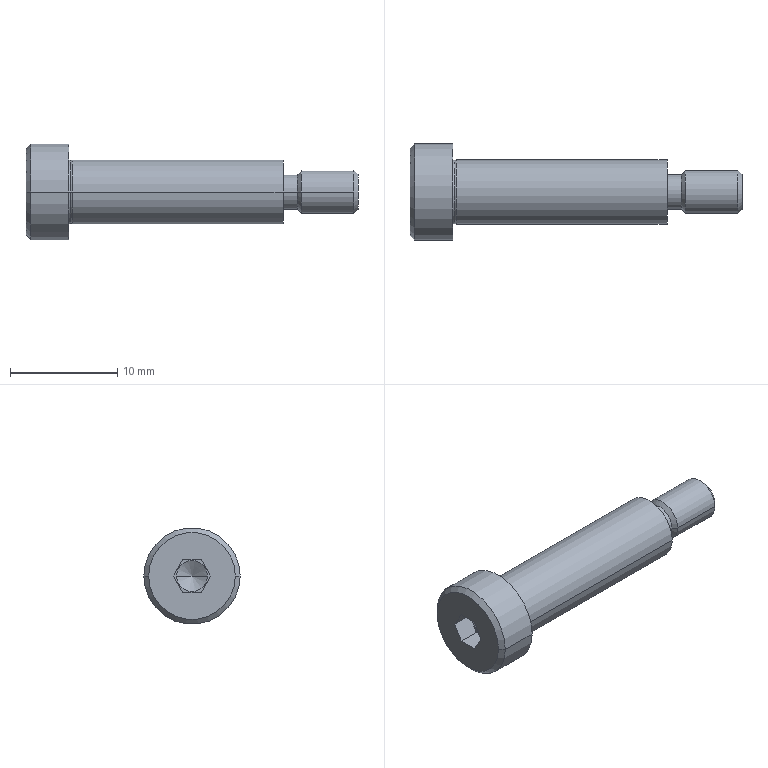Part | STEP file | 11-MSB6_2011 | 1 solid | 31 faces | box 31 x 9 x 9 mm | volume 880.105 mm3 | plane 11 | cone 8 | cylinder 8 | torus 4 | commonest cylinder face diameters 3.242 x2 4 x2 6 x2 9 x2
STEP:
#1=CARTESIAN_POINT('',(0.,-3.,0.));
#2=VERTEX_POINT('',#1);
#3=CARTESIAN_POINT('',(0.16,-2.956,0.));
#4=VERTEX_POINT('',#3);
#5=CARTESIAN_POINT('',(0.16,-3.271,0.));
#6=DIRECTION('',(0.,0.,-1.));
#7=DIRECTION('',(-1.,0.,0.));
#8=AXIS2_PLACEMENT_3D('',#5,#6,#7);
#9=CIRCLE('',#8,0.315);
#10=EDGE_CURVE('',#2,#4,#9,.T.);
#11=ORIENTED_EDGE('',*,*,#10,.T.);
#12=CARTESIAN_POINT('',(0.16,2.956,0.));
#13=VERTEX_POINT('',#12);
#14=CARTESIAN_POINT('',(0.16,0.,0.));
#15=DIRECTION('',(-1.,0.,0.));
#16=DIRECTION('',(0.,-1.,0.));
#17=AXIS2_PLACEMENT_3D('',#14,#15,#16);
#18=CIRCLE('',#17,2.956);
#19=EDGE_CURVE('',#4,#13,#18,.T.);
#20=ORIENTED_EDGE('',*,*,#19,.T.);
#21=CARTESIAN_POINT('',(0.,3.,0.));
#22=VERTEX_POINT('',#21);
#23=CARTESIAN_POINT('',(0.16,3.271,0.));
#24=DIRECTION('',(0.,0.,1.));
#25=DIRECTION('',(0.,-1.,0.));
#26=AXIS2_PLACEMENT_3D('',#23,#24,#25);
#27=CIRCLE('',#26,0.315);
#28=EDGE_CURVE('',#22,#13,#27,.T.);
#29=ORIENTED_EDGE('',*,*,#28,.F.);
#30=CARTESIAN_POINT('',(0.,0.,0.));
#31=DIRECTION('',(-1.,0.,0.));
#32=DIRECTION('',(0.,-1.,0.));
#33=AXIS2_PLACEMENT_3D('',#30,#31,#32);
#34=CIRCLE('',#33,3.);
#35=EDGE_CURVE('',#2,#22,#34,.T.);
#36=ORIENTED_EDGE('',*,*,#35,.F.);
#37=EDGE_LOOP('',(#11,#20,#29,#36));
#38=FACE_OUTER_BOUND('',#37,.T.);
#39=CARTESIAN_POINT('',(0.16,0.,0.));
#40=DIRECTION('',(-1.,0.,0.));
#41=DIRECTION('',(0.,-1.,0.));
#42=AXIS2_PLACEMENT_3D('',#39,#40,#41);
#43=TOROIDAL_SURFACE('',#42,3.271,0.315);
#44=ADVANCED_FACE('',(#38),#43,.F.);
#45=ORIENTED_EDGE('',*,*,#28,.T.);
#46=CARTESIAN_POINT('',(0.16,0.,0.));
#47=DIRECTION('',(-1.,0.,0.));
#48=DIRECTION('',(0.,-1.,0.));
#49=AXIS2_PLACEMENT_3D('',#46,#47,#48);
#50=CIRCLE('',#49,2.956);
#51=EDGE_CURVE('',#13,#4,#50,.T.);
#52=ORIENTED_EDGE('',*,*,#51,.T.);
#53=ORIENTED_EDGE('',*,*,#10,.F.);
#54=CARTESIAN_POINT('',(0.,0.,0.));
#55=DIRECTION('',(-1.,0.,0.));
#56=DIRECTION('',(0.,-1.,0.));
#57=AXIS2_PLACEMENT_3D('',#54,#55,#56);
#58=CIRCLE('',#57,3.);
#59=EDGE_CURVE('',#22,#2,#58,.T.);
#60=ORIENTED_EDGE('',*,*,#59,.F.);
#61=EDGE_LOOP('',(#45,#52,#53,#60));
#62=FACE_OUTER_BOUND('',#61,.T.);
#63=CARTESIAN_POINT('',(0.16,0.,0.));
#64=DIRECTION('',(-1.,0.,0.));
#65=DIRECTION('',(0.,-1.,0.));
#66=AXIS2_PLACEMENT_3D('',#63,#64,#65);
#67=TOROIDAL_SURFACE('',#66,3.271,0.315);
#68=ADVANCED_FACE('',(#62),#67,.F.);
#69=CARTESIAN_POINT('',(-1.169,0.,0.));
#70=VERTEX_POINT('',#69);
#71=CARTESIAN_POINT('',(-2.,-1.44,0.));
#72=VERTEX_POINT('',#71);
#73=CARTESIAN_POINT('',(-2.,-1.44,0.));
#74=DIRECTION('',(-0.5,-0.866,0.));
#75=VECTOR('',#74,1000.);
#76=LINE('',#73,#75);
#77=EDGE_CURVE('',#70,#72,#76,.T.);
#78=ORIENTED_EDGE('',*,*,#77,.F.);
#79=CARTESIAN_POINT('',(-2.,1.44,0.));
#80=VERTEX_POINT('',#79);
#81=CARTESIAN_POINT('',(-2.,1.44,0.));
#82=DIRECTION('',(-0.5,0.866,0.));
#83=VECTOR('',#82,1000.);
#84=LINE('',#81,#83);
#85=EDGE_CURVE('',#70,#80,#84,.T.);
#86=ORIENTED_EDGE('',*,*,#85,.T.);
#87=CARTESIAN_POINT('',(-2.,0.,0.));
#88=DIRECTION('',(-1.,0.,0.));
#89=DIRECTION('',(0.,0.,-1.));
#90=AXIS2_PLACEMENT_3D('',#87,#88,#89);
#91=CIRCLE('',#90,1.44);
#92=EDGE_CURVE('',#80,#72,#91,.T.);
#93=ORIENTED_EDGE('',*,*,#92,.T.);
#94=EDGE_LOOP('',(#78,#86,#93));
#95=FACE_OUTER_BOUND('',#94,.T.);
#96=CARTESIAN_POINT('',(-2.,0.,0.));
#97=DIRECTION('',(-1.,0.,0.));
#98=DIRECTION('',(0.,-1.,0.));
#99=AXIS2_PLACEMENT_3D('',#96,#97,#98);
#100=CONICAL_SURFACE('',#99,1.44,1.047);
#101=ADVANCED_FACE('',(#95),#100,.F.);
#102=CARTESIAN_POINT('',(-4.,-4.05,0.));
#103=VERTEX_POINT('',#102);
#104=CARTESIAN_POINT('',(-4.,4.05,0.));
#105=VERTEX_POINT('',#104);
#106=CARTESIAN_POINT('',(-4.,0.,0.));
#107=DIRECTION('',(-1.,0.,0.));
#108=DIRECTION('',(0.,-1.,0.));
#109=AXIS2_PLACEMENT_3D('',#106,#107,#108);
#110=CIRCLE('',#109,4.05);
#111=EDGE_CURVE('',#103,#105,#110,.T.);
#112=ORIENTED_EDGE('',*,*,#111,.F.);
#113=CARTESIAN_POINT('',(-3.55,-4.5,0.));
#114=VERTEX_POINT('',#113);
#115=CARTESIAN_POINT('',(-3.55,-4.5,0.));
#116=DIRECTION('',(0.7071,-0.7071,0.));
#117=VECTOR('',#116,1000.);
#118=LINE('',#115,#117);
#119=EDGE_CURVE('',#103,#114,#118,.T.);
#120=ORIENTED_EDGE('',*,*,#119,.T.);
#121=CARTESIAN_POINT('',(-3.55,4.5,0.));
#122=VERTEX_POINT('',#121);
#123=CARTESIAN_POINT('',(-3.55,0.,0.));
#124=DIRECTION('',(-1.,0.,0.));
#125=DIRECTION('',(0.,-1.,0.));
#126=AXIS2_PLACEMENT_3D('',#123,#124,#125);
#127=CIRCLE('',#126,4.5);
#128=EDGE_CURVE('',#114,#122,#127,.T.);
#129=ORIENTED_EDGE('',*,*,#128,.T.);
#130=CARTESIAN_POINT('',(-3.55,4.5,0.));
#131=DIRECTION('',(0.7071,0.7071,0.));
#132=VECTOR('',#131,1000.);
#133=LINE('',#130,#132);
#134=EDGE_CURVE('',#105,#122,#133,.T.);
#135=ORIENTED_EDGE('',*,*,#134,.F.);
#136=EDGE_LOOP('',(#112,#120,#129,#135));
#137=FACE_OUTER_BOUND('',#136,.T.);
#138=CARTESIAN_POINT('',(-3.55,0.,0.));
#139=DIRECTION('',(1.,0.,0.));
#140=DIRECTION('',(0.,1.,0.));
#141=AXIS2_PLACEMENT_3D('',#138,#139,#140);
#142=CONICAL_SURFACE('',#141,4.5,0.7854);
#143=ADVANCED_FACE('',(#137),#142,.T.);
#144=CARTESIAN_POINT('',(0.,-4.5,0.));
#145=VERTEX_POINT('',#144);
#146=CARTESIAN_POINT('',(0.,4.5,0.));
#147=VERTEX_POINT('',#146);
#148=CARTESIAN_POINT('',(0.,0.,0.));
#149=DIRECTION('',(-1.,0.,0.));
#150=DIRECTION('',(0.,-1.,0.));
#151=AXIS2_PLACEMENT_3D('',#148,#149,#150);
#152=CIRCLE('',#151,4.5);
#153=EDGE_CURVE('',#145,#147,#152,.T.);
#154=ORIENTED_EDGE('',*,*,#153,.T.);
#155=CARTESIAN_POINT('',(27.,4.5,0.));
#156=DIRECTION('',(-1.,0.,0.));
#157=VECTOR('',#156,1000.);
#158=LINE('',#155,#157);
#159=EDGE_CURVE('',#147,#122,#158,.T.);
#160=ORIENTED_EDGE('',*,*,#159,.T.);
#161=ORIENTED_EDGE('',*,*,#128,.F.);
#162=CARTESIAN_POINT('',(27.,-4.5,0.));
#163=DIRECTION('',(-1.,0.,0.));
#164=VECTOR('',#163,1000.);
#165=LINE('',#162,#164);
#166=EDGE_CURVE('',#145,#114,#165,.T.);
#167=ORIENTED_EDGE('',*,*,#166,.F.);
#168=EDGE_LOOP('',(#154,#160,#161,#167));
#169=FACE_OUTER_BOUND('',#168,.T.);
#170=CARTESIAN_POINT('',(27.,0.,0.));
#171=DIRECTION('',(-1.,0.,0.));
#172=DIRECTION('',(0.,-1.,0.));
#173=AXIS2_PLACEMENT_3D('',#170,#171,#172);
#174=CYLINDRICAL_SURFACE('',#173,4.5);
#175=ADVANCED_FACE('',(#169),#174,.T.);
#176=ORIENTED_EDGE('',*,*,#51,.F.);
#177=CARTESIAN_POINT('',(0.32,3.,0.));
#178=VERTEX_POINT('',#177);
#179=CARTESIAN_POINT('',(0.16,3.271,0.));
#180=DIRECTION('',(0.,0.,1.));
#181=DIRECTION('',(0.,-1.,0.));
#182=AXIS2_PLACEMENT_3D('',#179,#180,#181);
#183=CIRCLE('',#182,0.315);
#184=EDGE_CURVE('',#13,#178,#183,.T.);
#185=ORIENTED_EDGE('',*,*,#184,.T.);
#186=CARTESIAN_POINT('',(0.32,-3.,0.));
#187=VERTEX_POINT('',#186);
#188=CARTESIAN_POINT('',(0.32,0.,0.));
#189=DIRECTION('',(-1.,0.,0.));
#190=DIRECTION('',(0.,-1.,0.));
#191=AXIS2_PLACEMENT_3D('',#188,#189,#190);
#192=CIRCLE('',#191,3.);
#193=EDGE_CURVE('',#178,#187,#192,.T.);
#194=ORIENTED_EDGE('',*,*,#193,.T.);
#195=CARTESIAN_POINT('',(0.16,-3.271,0.));
#196=DIRECTION('',(0.,0.,-1.));
#197=DIRECTION('',(-1.,0.,0.));
#198=AXIS2_PLACEMENT_3D('',#195,#196,#197);
#199=CIRCLE('',#198,0.315);
#200=EDGE_CURVE('',#4,#187,#199,.T.);
#201=ORIENTED_EDGE('',*,*,#200,.F.);
#202=EDGE_LOOP('',(#176,#185,#194,#201));
#203=FACE_OUTER_BOUND('',#202,.T.);
#204=CARTESIAN_POINT('',(0.16,0.,0.));
#205=DIRECTION('',(-1.,0.,0.));
#206=DIRECTION('',(0.,-1.,0.));
#207=AXIS2_PLACEMENT_3D('',#204,#205,#206);
#208=TOROIDAL_SURFACE('',#207,3.271,0.315);
#209=ADVANCED_FACE('',(#203),#208,.F.);
#210=CARTESIAN_POINT('',(20.,-3.,0.));
#211=VERTEX_POINT('',#210);
#212=CARTESIAN_POINT('',(20.,3.,0.));
#213=VERTEX_POINT('',#212);
#214=CARTESIAN_POINT('',(20.,0.,0.));
#215=DIRECTION('',(-1.,0.,0.));
#216=DIRECTION('',(0.,-1.,0.));
#217=AXIS2_PLACEMENT_3D('',#214,#215,#216);
#218=CIRCLE('',#217,3.);
#219=EDGE_CURVE('',#211,#213,#218,.T.);
#220=ORIENTED_EDGE('',*,*,#219,.T.);
#221=CARTESIAN_POINT('',(27.,3.,0.));
#222=DIRECTION('',(-1.,0.,0.));
#223=VECTOR('',#222,1000.);
#224=LINE('',#221,#223);
#225=EDGE_CURVE('',#213,#178,#224,.T.);
#226=ORIENTED_EDGE('',*,*,#225,.T.);
#227=CARTESIAN_POINT('',(0.32,0.,0.));
#228=DIRECTION('',(-1.,0.,0.));
#229=DIRECTION('',(0.,-1.,0.));
#230=AXIS2_PLACEMENT_3D('',#227,#228,#229);
#231=CIRCLE('',#230,3.);
#232=EDGE_CURVE('',#187,#178,#231,.T.);
#233=ORIENTED_EDGE('',*,*,#232,.F.);
#234=CARTESIAN_POINT('',(27.,-3.,0.));
#235=DIRECTION('',(-1.,0.,0.));
#236=VECTOR('',#235,1000.);
#237=LINE('',#234,#236);
#238=EDGE_CURVE('',#211,#187,#237,.T.);
#239=ORIENTED_EDGE('',*,*,#238,.F.);
#240=EDGE_LOOP('',(#220,#226,#233,#239));
#241=FACE_OUTER_BOUND('',#240,.T.);
#242=CARTESIAN_POINT('',(27.,0.,0.));
#243=DIRECTION('',(-1.,0.,0.));
#244=DIRECTION('',(0.,-1.,0.));
#245=AXIS2_PLACEMENT_3D('',#242,#243,#244);
#246=CYLINDRICAL_SURFACE('',#245,3.);
#247=ADVANCED_FACE('',(#241),#246,.T.);
#248=CARTESIAN_POINT('',(21.342,-1.621,0.));
#249=VERTEX_POINT('',#248);
#250=CARTESIAN_POINT('',(21.342,1.621,0.));
#251=VERTEX_POINT('',#250);
#252=CARTESIAN_POINT('',(21.342,0.,0.));
#253=DIRECTION('',(-1.,0.,0.));
#254=DIRECTION('',(0.,-1.,0.));
#255=AXIS2_PLACEMENT_3D('',#252,#253,#254);
#256=CIRCLE('',#255,1.621);
#257=EDGE_CURVE('',#249,#251,#256,.T.);
#258=ORIENTED_EDGE('',*,*,#257,.T.);
#259=CARTESIAN_POINT('',(20.,1.621,0.));
#260=VERTEX_POINT('',#259);
#261=CARTESIAN_POINT('',(27.,1.621,0.));
#262=DIRECTION('',(-1.,0.,0.));
#263=VECTOR('',#262,1000.);
#264=LINE('',#261,#263);
#265=EDGE_CURVE('',#251,#260,#264,.T.);
#266=ORIENTED_EDGE('',*,*,#265,.T.);
#267=CARTESIAN_POINT('',(20.,-1.621,0.));
#268=VERTEX_POINT('',#267);
#269=CARTESIAN_POINT('',(20.,0.,0.));
#270=DIRECTION('',(-1.,0.,0.));
#271=DIRECTION('',(0.,-1.,0.));
#272=AXIS2_PLACEMENT_3D('',#269,#270,#271);
#273=CIRCLE('',#272,1.621);
#274=EDGE_CURVE('',#268,#260,#273,.T.);
#275=ORIENTED_EDGE('',*,*,#274,.F.);
#276=CARTESIAN_POINT('',(27.,-1.621,0.));
#277=DIRECTION('',(-1.,0.,0.));
#278=VECTOR('',#277,1000.);
#279=LINE('',#276,#278);
#280=EDGE_CURVE('',#249,#268,#279,.T.);
#281=ORIENTED_EDGE('',*,*,#280,.F.);
#282=EDGE_LOOP('',(#258,#266,#275,#281));
#283=FACE_OUTER_BOUND('',#282,.T.);
#284=CARTESIAN_POINT('',(27.,0.,0.));
#285=DIRECTION('',(-1.,0.,0.));
#286=DIRECTION('',(0.,-1.,0.));
#287=AXIS2_PLACEMENT_3D('',#284,#285,#286);
#288=CYLINDRICAL_SURFACE('',#287,1.621);
#289=ADVANCED_FACE('',(#283),#288,.T.);
#290=ORIENTED_EDGE('',*,*,#257,.F.);
#291=CARTESIAN_POINT('',(21.721,-2.,0.));
#292=VERTEX_POINT('',#291);
#293=CARTESIAN_POINT('',(21.721,-2.,0.));
#294=DIRECTION('',(0.7071,-0.7071,0.));
#295=VECTOR('',#294,1000.);
#296=LINE('',#293,#295);
#297=EDGE_CURVE('',#249,#292,#296,.T.);
#298=ORIENTED_EDGE('',*,*,#297,.T.);
#299=CARTESIAN_POINT('',(21.721,2.,0.));
#300=VERTEX_POINT('',#299);
#301=CARTESIAN_POINT('',(21.721,0.,0.));
#302=DIRECTION('',(-1.,0.,0.));
#303=DIRECTION('',(0.,-1.,0.));
#304=AXIS2_PLACEMENT_3D('',#301,#302,#303);
#305=CIRCLE('',#304,2.);
#306=EDGE_CURVE('',#292,#300,#305,.T.);
#307=ORIENTED_EDGE('',*,*,#306,.T.);
#308=CARTESIAN_POINT('',(21.721,2.,0.));
#309=DIRECTION('',(0.7071,0.7071,0.));
#310=VECTOR('',#309,1000.);
#311=LINE('',#308,#310);
#312=EDGE_CURVE('',#251,#300,#311,.T.);
#313=ORIENTED_EDGE('',*,*,#312,.F.);
#314=EDGE_LOOP('',(#290,#298,#307,#313));
#315=FACE_OUTER_BOUND('',#314,.T.);
#316=CARTESIAN_POINT('',(21.721,0.,0.));
#317=DIRECTION('',(1.,0.,0.));
#318=DIRECTION('',(0.,1.,0.));
#319=AXIS2_PLACEMENT_3D('',#316,#317,#318);
#320=CONICAL_SURFACE('',#319,2.,0.7854);
#321=ADVANCED_FACE('',(#315),#320,.T.);
#322=CARTESIAN_POINT('',(26.621,-2.,0.));
#323=VERTEX_POINT('',#322);
#324=CARTESIAN_POINT('',(26.621,2.,0.));
#325=VERTEX_POINT('',#324);
#326=CARTESIAN_POINT('',(26.621,0.,0.));
#327=DIRECTION('',(-1.,0.,0.));
#328=DIRECTION('',(0.,-1.,0.));
#329=AXIS2_PLACEMENT_3D('',#326,#327,#328);
#330=CIRCLE('',#329,2.);
#331=EDGE_CURVE('',#323,#325,#330,.T.);
#332=ORIENTED_EDGE('',*,*,#331,.T.);
#333=CARTESIAN_POINT('',(27.,2.,0.));
#334=DIRECTION('',(-1.,0.,0.));
#335=VECTOR('',#334,1000.);
#336=LINE('',#333,#335);
#337=EDGE_CURVE('',#325,#300,#336,.T.);
#338=ORIENTED_EDGE('',*,*,#337,.T.);
#339=ORIENTED_EDGE('',*,*,#306,.F.);
#340=CARTESIAN_POINT('',(27.,-2.,0.));
#341=DIRECTION('',(-1.,0.,0.));
#342=VECTOR('',#341,1000.);
#343=LINE('',#340,#342);
#344=EDGE_CURVE('',#323,#292,#343,.T.);
#345=ORIENTED_EDGE('',*,*,#344,.F.);
#346=EDGE_LOOP('',(#332,#338,#339,#345));
#347=FACE_OUTER_BOUND('',#346,.T.);
#348=CARTESIAN_POINT('',(27.,0.,0.));
#349=DIRECTION('',(-1.,0.,0.));
#350=DIRECTION('',(0.,-1.,0.));
#351=AXIS2_PLACEMENT_3D('',#348,#349,#350);
#352=CYLINDRICAL_SURFACE('',#351,2.);
#353=ADVANCED_FACE('',(#347),#352,.T.);
#354=CARTESIAN_POINT('',(27.,-1.621,0.));
#355=VERTEX_POINT('',#354);
#356=CARTESIAN_POINT('',(27.,1.621,0.));
#357=VERTEX_POINT('',#356);
#358=CARTESIAN_POINT('',(27.,0.,0.));
#359=DIRECTION('',(-1.,0.,0.));
#360=DIRECTION('',(0.,-1.,0.));
#361=AXIS2_PLACEMENT_3D('',#358,#359,#360);
#362=CIRCLE('',#361,1.621);
#363=EDGE_CURVE('',#355,#357,#362,.T.);
#364=ORIENTED_EDGE('',*,*,#363,.T.);
#365=CARTESIAN_POINT('',(27.,1.621,0.));
#366=DIRECTION('',(-0.7071,0.7071,0.));
#367=VECTOR('',#366,1000.);
#368=LINE('',#365,#367);
#369=EDGE_CURVE('',#357,#325,#368,.T.);
#370=ORIENTED_EDGE('',*,*,#369,.T.);
#371=ORIENTED_EDGE('',*,*,#331,.F.);
#372=CARTESIAN_POINT('',(27.,-1.621,0.));
#373=DIRECTION('',(-0.7071,-0.7071,0.));
#374=VECTOR('',#373,1000.);
#375=LINE('',#372,#374);
#376=EDGE_CURVE('',#355,#323,#375,.T.);
#377=ORIENTED_EDGE('',*,*,#376,.F.);
#378=EDGE_LOOP('',(#364,#370,#371,#377));
#379=FACE_OUTER_BOUND('',#378,.T.);
#380=CARTESIAN_POINT('',(27.,0.,0.));
#381=DIRECTION('',(-1.,0.,0.));
#382=DIRECTION('',(0.,-1.,0.));
#383=AXIS2_PLACEMENT_3D('',#380,#381,#382);
#384=CONICAL_SURFACE('',#383,1.621,0.7854);
#385=ADVANCED_FACE('',(#379),#384,.T.);
#386=CARTESIAN_POINT('',(-4.,0.,0.));
#387=DIRECTION('',(-1.,0.,0.));
#388=DIRECTION('',(0.,-1.,0.));
#389=AXIS2_PLACEMENT_3D('',#386,#387,#388);
#390=CIRCLE('',#389,4.05);
#391=EDGE_CURVE('',#105,#103,#390,.T.);
#392=ORIENTED_EDGE('',*,*,#391,.T.);
#393=ORIENTED_EDGE('',*,*,#111,.T.);
#394=EDGE_LOOP('',(#392,#393));
#395=FACE_OUTER_BOUND('',#394,.T.);
#396=CARTESIAN_POINT('',(-4.,1.732,0.));
#397=VERTEX_POINT('',#396);
#398=CARTESIAN_POINT('',(-4.,0.866,1.5));
#399=VERTEX_POINT('',#398);
#400=CARTESIAN_POINT('',(-4.,1.732,0.));
#401=DIRECTION('',(0.,-0.5,0.866));
#402=VECTOR('',#401,1000.);
#403=LINE('',#400,#402);
#404=EDGE_CURVE('',#397,#399,#403,.T.);
#405=ORIENTED_EDGE('',*,*,#404,.T.);
#406=CARTESIAN_POINT('',(-4.,-0.866,1.5));
#407=VERTEX_POINT('',#406);
#408=CARTESIAN_POINT('',(-4.,0.866,1.5));
#409=DIRECTION('',(0.,-1.,0.));
#410=VECTOR('',#409,1000.);
#411=LINE('',#408,#410);
#412=EDGE_CURVE('',#399,#407,#411,.T.);
#413=ORIENTED_EDGE('',*,*,#412,.T.);
#414=CARTESIAN_POINT('',(-4.,-1.732,0.));
#415=VERTEX_POINT('',#414);
#416=CARTESIAN_POINT('',(-4.,-0.866,1.5));
#417=DIRECTION('',(0.,-0.5,-0.866));
#418=VECTOR('',#417,1000.);
#419=LINE('',#416,#418);
#420=EDGE_CURVE('',#407,#415,#419,.T.);
#421=ORIENTED_EDGE('',*,*,#420,.T.);
#422=CARTESIAN_POINT('',(-4.,-0.866,-1.5));
#423=VERTEX_POINT('',#422);
#424=CARTESIAN_POINT('',(-4.,-1.732,0.));
#425=DIRECTION('',(0.,0.5,-0.866));
#426=VECTOR('',#425,1000.);
#427=LINE('',#424,#426);
#428=EDGE_CURVE('',#415,#423,#427,.T.);
#429=ORIENTED_EDGE('',*,*,#428,.T.);
#430=CARTESIAN_POINT('',(-4.,0.866,-1.5));
#431=VERTEX_POINT('',#430);
#432=CARTESIAN_POINT('',(-4.,-0.866,-1.5));
#433=DIRECTION('',(0.,1.,0.));
#434=VECTOR('',#433,1000.);
#435=LINE('',#432,#434);
#436=EDGE_CURVE('',#423,#431,#435,.T.);
#437=ORIENTED_EDGE('',*,*,#436,.T.);
#438=CARTESIAN_POINT('',(-4.,0.866,-1.5));
#439=DIRECTION('',(0.,0.5,0.866));
#440=VECTOR('',#439,1000.);
#441=LINE('',#438,#440);
#442=EDGE_CURVE('',#431,#397,#441,.T.);
#443=ORIENTED_EDGE('',*,*,#442,.T.);
#444=EDGE_LOOP('',(#405,#413,#421,#429,#437,#443));
#445=FACE_BOUND('',#444,.T.);
#446=CARTESIAN_POINT('',(-4.,1.44,0.));
#447=DIRECTION('',(1.,0.,0.));
#448=DIRECTION('',(0.,1.,0.));
#449=AXIS2_PLACEMENT_3D('',#446,#447,#448);
#450=PLANE('',#449);
#451=ADVANCED_FACE('',(#395,#445),#450,.F.);
#452=ORIENTED_EDGE('',*,*,#363,.F.);
#453=CARTESIAN_POINT('',(27.,0.,0.));
#454=DIRECTION('',(-1.,0.,0.));
#455=DIRECTION('',(0.,-1.,0.));
#456=AXIS2_PLACEMENT_3D('',#453,#454,#455);
#457=CIRCLE('',#456,1.621);
#458=EDGE_CURVE('',#357,#355,#457,.T.);
#459=ORIENTED_EDGE('',*,*,#458,.F.);
#460=EDGE_LOOP('',(#452,#459));
#461=FACE_OUTER_BOUND('',#460,.T.);
#462=CARTESIAN_POINT('',(27.,1.621,0.));
#463=DIRECTION('',(-1.,0.,0.));
#464=DIRECTION('',(0.,-1.,0.));
#465=AXIS2_PLACEMENT_3D('',#462,#463,#464);
#466=PLANE('',#465);
#467=ADVANCED_FACE('',(#461),#466,.F.);
#468=ORIENTED_EDGE('',*,*,#369,.F.);
#469=ORIENTED_EDGE('',*,*,#458,.T.);
#470=ORIENTED_EDGE('',*,*,#376,.T.);
#471=CARTESIAN_POINT('',(26.621,0.,0.));
#472=DIRECTION('',(-1.,0.,0.));
#473=DIRECTION('',(0.,-1.,0.));
#474=AXIS2_PLACEMENT_3D('',#471,#472,#473);
#475=CIRCLE('',#474,2.);
#476=EDGE_CURVE('',#325,#323,#475,.T.);
#477=ORIENTED_EDGE('',*,*,#476,.F.);
#478=EDGE_LOOP('',(#468,#469,#470,#477));
#479=FACE_OUTER_BOUND('',#478,.T.);
#480=CARTESIAN_POINT('',(27.,0.,0.));
#481=DIRECTION('',(-1.,0.,0.));
#482=DIRECTION('',(0.,-1.,0.));
#483=AXIS2_PLACEMENT_3D('',#480,#481,#482);
#484=CONICAL_SURFACE('',#483,1.621,0.7854);
#485=ADVANCED_FACE('',(#479),#484,.T.);
#486=ORIENTED_EDGE('',*,*,#337,.F.);
#487=ORIENTED_EDGE('',*,*,#476,.T.);
#488=ORIENTED_EDGE('',*,*,#344,.T.);
#489=CARTESIAN_POINT('',(21.721,0.,0.));
#490=DIRECTION('',(-1.,0.,0.));
#491=DIRECTION('',(0.,-1.,0.));
#492=AXIS2_PLACEMENT_3D('',#489,#490,#491);
#493=CIRCLE('',#492,2.);
#494=EDGE_CURVE('',#300,#292,#493,.T.);
#495=ORIENTED_EDGE('',*,*,#494,.F.);
#496=EDGE_LOOP('',(#486,#487,#488,#495));
#497=FACE_OUTER_BOUND('',#496,.T.);
#498=CARTESIAN_POINT('',(27.,0.,0.));
#499=DIRECTION('',(-1.,0.,0.));
#500=DIRECTION('',(0.,-1.,0.));
#501=AXIS2_PLACEMENT_3D('',#498,#499,#500);
#502=CYLINDRICAL_SURFACE('',#501,2.);
#503=ADVANCED_FACE('',(#497),#502,.T.);
#504=ORIENTED_EDGE('',*,*,#297,.F.);
#505=CARTESIAN_POINT('',(21.342,0.,0.));
#506=DIRECTION('',(-1.,0.,0.));
#507=DIRECTION('',(0.,-1.,0.));
#508=AXIS2_PLACEMENT_3D('',#505,#506,#507);
#509=CIRCLE('',#508,1.621);
#510=EDGE_CURVE('',#251,#249,#509,.T.);
#511=ORIENTED_EDGE('',*,*,#510,.F.);
#512=ORIENTED_EDGE('',*,*,#312,.T.);
#513=ORIENTED_EDGE('',*,*,#494,.T.);
#514=EDGE_LOOP('',(#504,#511,#512,#513));
#515=FACE_OUTER_BOUND('',#514,.T.);
#516=CARTESIAN_POINT('',(21.721,0.,0.));
#517=DIRECTION('',(1.,0.,0.));
#518=DIRECTION('',(0.,1.,0.));
#519=AXIS2_PLACEMENT_3D('',#516,#517,#518);
#520=CONICAL_SURFACE('',#519,2.,0.7854);
#521=ADVANCED_FACE('',(#515),#520,.T.);
#522=ORIENTED_EDGE('',*,*,#265,.F.);
#523=ORIENTED_EDGE('',*,*,#510,.T.);
#524=ORIENTED_EDGE('',*,*,#280,.T.);
#525=CARTESIAN_POINT('',(20.,0.,0.));
#526=DIRECTION('',(-1.,0.,0.));
#527=DIRECTION('',(0.,-1.,0.));
#528=AXIS2_PLACEMENT_3D('',#525,#526,#527);
#529=CIRCLE('',#528,1.621);
#530=EDGE_CURVE('',#260,#268,#529,.T.);
#531=ORIENTED_EDGE('',*,*,#530,.F.);
#532=EDGE_LOOP('',(#522,#523,#524,#531));
#533=FACE_OUTER_BOUND('',#532,.T.);
#534=CARTESIAN_POINT('',(27.,0.,0.));
#535=DIRECTION('',(-1.,0.,0.));
#536=DIRECTION('',(0.,-1.,0.));
#537=AXIS2_PLACEMENT_3D('',#534,#535,#536);
#538=CYLINDRICAL_SURFACE('',#537,1.621);
#539=ADVANCED_FACE('',(#533),#538,.T.);
#540=ORIENTED_EDGE('',*,*,#219,.F.);
#541=CARTESIAN_POINT('',(20.,0.,0.));
#542=DIRECTION('',(-1.,0.,0.));
#543=DIRECTION('',(0.,-1.,0.));
#544=AXIS2_PLACEMENT_3D('',#541,#542,#543);
#545=CIRCLE('',#544,3.);
#546=EDGE_CURVE('',#213,#211,#545,.T.);
#547=ORIENTED_EDGE('',*,*,#546,.F.);
#548=EDGE_LOOP('',(#540,#547));
#549=FACE_OUTER_BOUND('',#548,.T.);
#550=ORIENTED_EDGE('',*,*,#274,.T.);
#551=ORIENTED_EDGE('',*,*,#530,.T.);
#552=EDGE_LOOP('',(#550,#551));
#553=FACE_BOUND('',#552,.T.);
#554=CARTESIAN_POINT('',(20.,3.,0.));
#555=DIRECTION('',(-1.,0.,0.));
#556=DIRECTION('',(0.,-1.,0.));
#557=AXIS2_PLACEMENT_3D('',#554,#555,#556);
#558=PLANE('',#557);
#559=ADVANCED_FACE('',(#549,#553),#558,.F.);
#560=ORIENTED_EDGE('',*,*,#225,.F.);
#561=ORIENTED_EDGE('',*,*,#546,.T.);
#562=ORIENTED_EDGE('',*,*,#238,.T.);
#563=ORIENTED_EDGE('',*,*,#193,.F.);
#564=EDGE_LOOP('',(#560,#561,#562,#563));
#565=FACE_OUTER_BOUND('',#564,.T.);
#566=CARTESIAN_POINT('',(27.,0.,0.));
#567=DIRECTION('',(-1.,0.,0.));
#568=DIRECTION('',(0.,-1.,0.));
#569=AXIS2_PLACEMENT_3D('',#566,#567,#568);
#570=CYLINDRICAL_SURFACE('',#569,3.);
#571=ADVANCED_FACE('',(#565),#570,.T.);
#572=ORIENTED_EDGE('',*,*,#19,.F.);
#573=ORIENTED_EDGE('',*,*,#200,.T.);
#574=ORIENTED_EDGE('',*,*,#232,.T.);
#575=ORIENTED_EDGE('',*,*,#184,.F.);
#576=EDGE_LOOP('',(#572,#573,#574,#575));
#577=FACE_OUTER_BOUND('',#576,.T.);
#578=CARTESIAN_POINT('',(0.16,0.,0.));
#579=DIRECTION('',(-1.,0.,0.));
#580=DIRECTION('',(0.,-1.,0.));
#581=AXIS2_PLACEMENT_3D('',#578,#579,#580);
#582=TOROIDAL_SURFACE('',#581,3.271,0.315);
#583=ADVANCED_FACE('',(#577),#582,.F.);
#584=ORIENTED_EDGE('',*,*,#153,.F.);
#585=CARTESIAN_POINT('',(0.,0.,0.));
#586=DIRECTION('',(-1.,0.,0.));
#587=DIRECTION('',(0.,-1.,0.));
#588=AXIS2_PLACEMENT_3D('',#585,#586,#587);
#589=CIRCLE('',#588,4.5);
#590=EDGE_CURVE('',#147,#145,#589,.T.);
#591=ORIENTED_EDGE('',*,*,#590,.F.);
#592=EDGE_LOOP('',(#584,#591));
#593=FACE_OUTER_BOUND('',#592,.T.);
#594=ORIENTED_EDGE('',*,*,#35,.T.);
#595=ORIENTED_EDGE('',*,*,#59,.T.);
#596=EDGE_LOOP('',(#594,#595));
#597=FACE_BOUND('',#596,.T.);
#598=CARTESIAN_POINT('',(0.,4.5,0.));
#599=DIRECTION('',(-1.,0.,0.));
#600=DIRECTION('',(0.,-1.,0.));
#601=AXIS2_PLACEMENT_3D('',#598,#599,#600);
#602=PLANE('',#601);
#603=ADVANCED_FACE('',(#593,#597),#602,.F.);
#604=ORIENTED_EDGE('',*,*,#159,.F.);
#605=ORIENTED_EDGE('',*,*,#590,.T.);
#606=ORIENTED_EDGE('',*,*,#166,.T.);
#607=CARTESIAN_POINT('',(-3.55,0.,0.));
#608=DIRECTION('',(-1.,0.,0.));
#609=DIRECTION('',(0.,-1.,0.));
#610=AXIS2_PLACEMENT_3D('',#607,#608,#609);
#611=CIRCLE('',#610,4.5);
#612=EDGE_CURVE('',#122,#114,#611,.T.);
#613=ORIENTED_EDGE('',*,*,#612,.F.);
#614=EDGE_LOOP('',(#604,#605,#606,#613));
#615=FACE_OUTER_BOUND('',#614,.T.);
#616=CARTESIAN_POINT('',(27.,0.,0.));
#617=DIRECTION('',(-1.,0.,0.));
#618=DIRECTION('',(0.,-1.,0.));
#619=AXIS2_PLACEMENT_3D('',#616,#617,#618);
#620=CYLINDRICAL_SURFACE('',#619,4.5);
#621=ADVANCED_FACE('',(#615),#620,.T.);
#622=ORIENTED_EDGE('',*,*,#119,.F.);
#623=ORIENTED_EDGE('',*,*,#391,.F.);
#624=ORIENTED_EDGE('',*,*,#134,.T.);
#625=ORIENTED_EDGE('',*,*,#612,.T.);
#626=EDGE_LOOP('',(#622,#623,#624,#625));
#627=FACE_OUTER_BOUND('',#626,.T.);
#628=CARTESIAN_POINT('',(-3.55,0.,0.));
#629=DIRECTION('',(1.,0.,0.));
#630=DIRECTION('',(0.,1.,0.));
#631=AXIS2_PLACEMENT_3D('',#628,#629,#630);
#632=CONICAL_SURFACE('',#631,4.5,0.7854);
#633=ADVANCED_FACE('',(#627),#632,.T.);
#634=CARTESIAN_POINT('',(-2.,1.732,0.));
#635=VERTEX_POINT('',#634);
#636=CARTESIAN_POINT('',(-2.,0.866,1.5));
#637=VERTEX_POINT('',#636);
#638=CARTESIAN_POINT('',(-2.,1.732,0.));
#639=DIRECTION('',(0.,-0.5,0.866));
#640=VECTOR('',#639,1000.);
#641=LINE('',#638,#640);
#642=EDGE_CURVE('',#635,#637,#641,.T.);
#643=ORIENTED_EDGE('',*,*,#642,.F.);
#644=CARTESIAN_POINT('',(-2.,0.866,-1.5));
#645=VERTEX_POINT('',#644);
#646=CARTESIAN_POINT('',(-2.,0.866,-1.5));
#647=DIRECTION('',(0.,0.5,0.866));
#648=VECTOR('',#647,1000.);
#649=LINE('',#646,#648);
#650=EDGE_CURVE('',#645,#635,#649,.T.);
#651=ORIENTED_EDGE('',*,*,#650,.F.);
#652=CARTESIAN_POINT('',(-2.,-0.866,-1.5));
#653=VERTEX_POINT('',#652);
#654=CARTESIAN_POINT('',(-2.,-0.866,-1.5));
#655=DIRECTION('',(0.,1.,0.));
#656=VECTOR('',#655,1000.);
#657=LINE('',#654,#656);
#658=EDGE_CURVE('',#653,#645,#657,.T.);
#659=ORIENTED_EDGE('',*,*,#658,.F.);
#660=CARTESIAN_POINT('',(-2.,-1.732,0.));
#661=VERTEX_POINT('',#660);
#662=CARTESIAN_POINT('',(-2.,-1.732,0.));
#663=DIRECTION('',(0.,0.5,-0.866));
#664=VECTOR('',#663,1000.);
#665=LINE('',#662,#664);
#666=EDGE_CURVE('',#661,#653,#665,.T.);
#667=ORIENTED_EDGE('',*,*,#666,.F.);
#668=CARTESIAN_POINT('',(-2.,-0.866,1.5));
#669=VERTEX_POINT('',#668);
#670=CARTESIAN_POINT('',(-2.,-0.866,1.5));
#671=DIRECTION('',(0.,-0.5,-0.866));
#672=VECTOR('',#671,1000.);
#673=LINE('',#670,#672);
#674=EDGE_CURVE('',#669,#661,#673,.T.);
#675=ORIENTED_EDGE('',*,*,#674,.F.);
#676=CARTESIAN_POINT('',(-2.,0.866,1.5));
#677=DIRECTION('',(0.,-1.,0.));
#678=VECTOR('',#677,1000.);
#679=LINE('',#676,#678);
#680=EDGE_CURVE('',#637,#669,#679,.T.);
#681=ORIENTED_EDGE('',*,*,#680,.F.);
#682=EDGE_LOOP('',(#643,#651,#659,#667,#675,#681));
#683=FACE_OUTER_BOUND('',#682,.T.);
#684=CARTESIAN_POINT('',(-2.,0.,0.));
#685=DIRECTION('',(-1.,0.,0.));
#686=DIRECTION('',(0.,0.,-1.));
#687=AXIS2_PLACEMENT_3D('',#684,#685,#686);
#688=CIRCLE('',#687,1.44);
#689=EDGE_CURVE('',#72,#80,#688,.T.);
#690=ORIENTED_EDGE('',*,*,#689,.F.);
#691=ORIENTED_EDGE('',*,*,#92,.F.);
#692=EDGE_LOOP('',(#690,#691));
#693=FACE_BOUND('',#692,.T.);
#694=CARTESIAN_POINT('',(-2.,0.866,1.5));
#695=DIRECTION('',(1.,0.,0.));
#696=DIRECTION('',(0.,0.,-1.));
#697=AXIS2_PLACEMENT_3D('',#694,#695,#696);
#698=PLANE('',#697);
#699=ADVANCED_FACE('',(#683,#693),#698,.F.);
#700=ORIENTED_EDGE('',*,*,#404,.F.);
#701=CARTESIAN_POINT('',(-2.,1.732,0.));
#702=DIRECTION('',(-1.,0.,0.));
#703=VECTOR('',#702,1000.);
#704=LINE('',#701,#703);
#705=EDGE_CURVE('',#635,#397,#704,.T.);
#706=ORIENTED_EDGE('',*,*,#705,.F.);
#707=ORIENTED_EDGE('',*,*,#642,.T.);
#708=CARTESIAN_POINT('',(-2.,0.866,1.5));
#709=DIRECTION('',(-1.,0.,0.));
#710=VECTOR('',#709,1000.);
#711=LINE('',#708,#710);
#712=EDGE_CURVE('',#637,#399,#711,.T.);
#713=ORIENTED_EDGE('',*,*,#712,.T.);
#714=EDGE_LOOP('',(#700,#706,#707,#713));
#715=FACE_OUTER_BOUND('',#714,.T.);
#716=CARTESIAN_POINT('',(-2.,1.732,0.));
#717=DIRECTION('',(0.,-0.866,-0.5));
#718=DIRECTION('',(0.,0.5,-0.866));
#719=AXIS2_PLACEMENT_3D('',#716,#717,#718);
#720=PLANE('',#719);
#721=ADVANCED_FACE('',(#715),#720,.T.);
#722=ORIENTED_EDGE('',*,*,#412,.F.);
#723=ORIENTED_EDGE('',*,*,#712,.F.);
#724=ORIENTED_EDGE('',*,*,#680,.T.);
#725=CARTESIAN_POINT('',(-2.,-0.866,1.5));
#726=DIRECTION('',(-1.,0.,0.));
#727=VECTOR('',#726,1000.);
#728=LINE('',#725,#727);
#729=EDGE_CURVE('',#669,#407,#728,.T.);
#730=ORIENTED_EDGE('',*,*,#729,.T.);
#731=EDGE_LOOP('',(#722,#723,#724,#730));
#732=FACE_OUTER_BOUND('',#731,.T.);
#733=CARTESIAN_POINT('',(-2.,0.866,1.5));
#734=DIRECTION('',(0.,0.,-1.));
#735=DIRECTION('',(-1.,0.,0.));
#736=AXIS2_PLACEMENT_3D('',#733,#734,#735);
#737=PLANE('',#736);
#738=ADVANCED_FACE('',(#732),#737,.T.);
#739=ORIENTED_EDGE('',*,*,#420,.F.);
#740=ORIENTED_EDGE('',*,*,#729,.F.);
#741=ORIENTED_EDGE('',*,*,#674,.T.);
#742=CARTESIAN_POINT('',(-2.,-1.732,0.));
#743=DIRECTION('',(-1.,0.,0.));
#744=VECTOR('',#743,1000.);
#745=LINE('',#742,#744);
#746=EDGE_CURVE('',#661,#415,#745,.T.);
#747=ORIENTED_EDGE('',*,*,#746,.T.);
#748=EDGE_LOOP('',(#739,#740,#741,#747));
#749=FACE_OUTER_BOUND('',#748,.T.);
#750=CARTESIAN_POINT('',(-2.,-0.866,1.5));
#751=DIRECTION('',(0.,0.866,-0.5));
#752=DIRECTION('',(0.,0.5,0.866));
#753=AXIS2_PLACEMENT_3D('',#750,#751,#752);
#754=PLANE('',#753);
#755=ADVANCED_FACE('',(#749),#754,.T.);
#756=ORIENTED_EDGE('',*,*,#428,.F.);
#757=ORIENTED_EDGE('',*,*,#746,.F.);
#758=ORIENTED_EDGE('',*,*,#666,.T.);
#759=CARTESIAN_POINT('',(-2.,-0.866,-1.5));
#760=DIRECTION('',(-1.,0.,0.));
#761=VECTOR('',#760,1000.);
#762=LINE('',#759,#761);
#763=EDGE_CURVE('',#653,#423,#762,.T.);
#764=ORIENTED_EDGE('',*,*,#763,.T.);
#765=EDGE_LOOP('',(#756,#757,#758,#764));
#766=FACE_OUTER_BOUND('',#765,.T.);
#767=CARTESIAN_POINT('',(-2.,-1.732,0.));
#768=DIRECTION('',(0.,0.866,0.5));
#769=DIRECTION('',(0.,-0.5,0.866));
#770=AXIS2_PLACEMENT_3D('',#767,#768,#769);
#771=PLANE('',#770);
#772=ADVANCED_FACE('',(#766),#771,.T.);
#773=ORIENTED_EDGE('',*,*,#436,.F.);
#774=ORIENTED_EDGE('',*,*,#763,.F.);
#775=ORIENTED_EDGE('',*,*,#658,.T.);
#776=CARTESIAN_POINT('',(-2.,0.866,-1.5));
#777=DIRECTION('',(-1.,0.,0.));
#778=VECTOR('',#777,1000.);
#779=LINE('',#776,#778);
#780=EDGE_CURVE('',#645,#431,#779,.T.);
#781=ORIENTED_EDGE('',*,*,#780,.T.);
#782=EDGE_LOOP('',(#773,#774,#775,#781));
#783=FACE_OUTER_BOUND('',#782,.T.);
#784=CARTESIAN_POINT('',(-2.,-0.866,-1.5));
#785=DIRECTION('',(0.,0.,1.));
#786=DIRECTION('',(1.,0.,0.));
#787=AXIS2_PLACEMENT_3D('',#784,#785,#786);
#788=PLANE('',#787);
#789=ADVANCED_FACE('',(#783),#788,.T.);
#790=ORIENTED_EDGE('',*,*,#442,.F.);
#791=ORIENTED_EDGE('',*,*,#780,.F.);
#792=ORIENTED_EDGE('',*,*,#650,.T.);
#793=ORIENTED_EDGE('',*,*,#705,.T.);
#794=EDGE_LOOP('',(#790,#791,#792,#793));
#795=FACE_OUTER_BOUND('',#794,.T.);
#796=CARTESIAN_POINT('',(-2.,0.866,-1.5));
#797=DIRECTION('',(0.,-0.866,0.5));
#798=DIRECTION('',(0.,-0.5,-0.866));
#799=AXIS2_PLACEMENT_3D('',#796,#797,#798);
#800=PLANE('',#799);
#801=ADVANCED_FACE('',(#795),#800,.T.);
#802=ORIENTED_EDGE('',*,*,#85,.F.);
#803=ORIENTED_EDGE('',*,*,#77,.T.);
#804=ORIENTED_EDGE('',*,*,#689,.T.);
#805=EDGE_LOOP('',(#802,#803,#804));
#806=FACE_OUTER_BOUND('',#805,.T.);
#807=CARTESIAN_POINT('',(-2.,0.,0.));
#808=DIRECTION('',(-1.,0.,0.));
#809=DIRECTION('',(0.,-1.,0.));
#810=AXIS2_PLACEMENT_3D('',#807,#808,#809);
#811=CONICAL_SURFACE('',#810,1.44,1.047);
#812=ADVANCED_FACE('',(#806),#811,.F.);
#813=CLOSED_SHELL('',(#44,#68,#101,#143,#175,#209,#247,#289,#321,#353,#385,#451,#467,#485,#503,#521,#539,#559,#571,#583,#603,#621,#633,#699,#721,#738,#755,#772,#789,#801,#812));
#814=MANIFOLD_SOLID_BREP('',#813);
#815=CARTESIAN_POINT('',(0.,0.,0.));
#816=DIRECTION('',(0.,0.,1.));
#817=DIRECTION('',(1.,0.,0.));
#818=AXIS2_PLACEMENT_3D('',#815,#816,#817);
#819=(LENGTH_UNIT()NAMED_UNIT(*)SI_UNIT(.MILLI.,.METRE.));
#820=UNCERTAINTY_MEASURE_WITH_UNIT(LENGTH_MEASURE(0.00001),#819,'','');
#821=(NAMED_UNIT(*)PLANE_ANGLE_UNIT()SI_UNIT($,.RADIAN.));
#822=(NAMED_UNIT(*)SI_UNIT($,.STERADIAN.)SOLID_ANGLE_UNIT());
#823=(GEOMETRIC_REPRESENTATION_CONTEXT(3)GLOBAL_UNCERTAINTY_ASSIGNED_CONTEXT((#820))GLOBAL_UNIT_ASSIGNED_CONTEXT((#819,#821,#822))REPRESENTATION_CONTEXT('',''));
#824=ADVANCED_BREP_SHAPE_REPRESENTATION('',(#814,#818),#823);